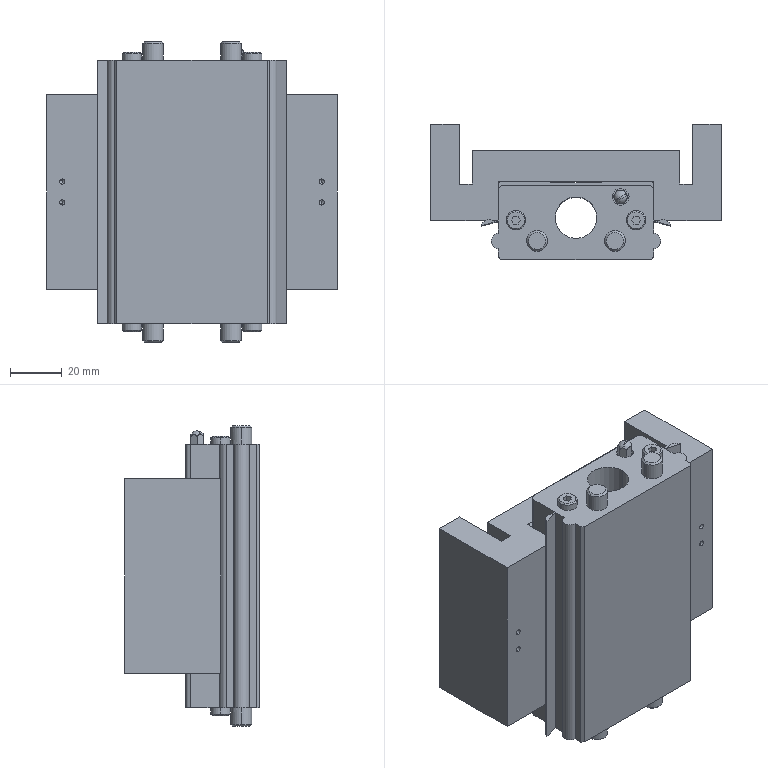Part | STEP file | Single-axis module KK8620C slider | 2 solids | 223 faces | box 112 x 52 x 116 mm | volume 327270 mm3 | plane 109 | cylinder 71 | cone 40 | sphere 3 | commonest cylinder face diameters 5 x20 6 x9 2.05 x8 7.5 x8 8 x8 2.15 x6